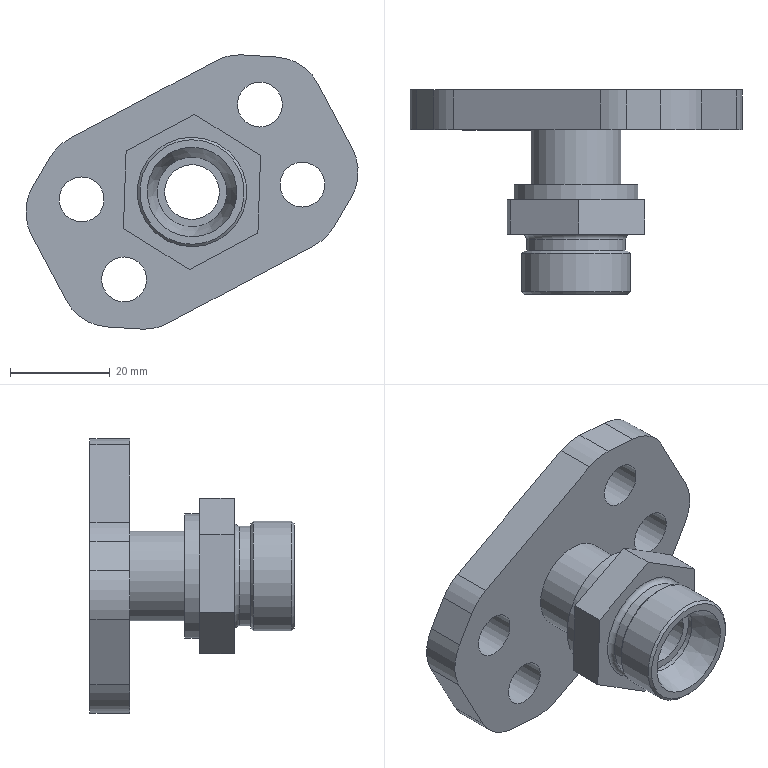Part | STEP file | HL4GZ-1.58.020 (cutter motor inlet/outlet flange) | 2 solids | 54 faces | box 66.692 x 41 x 55.077 mm | volume 25659 mm3 | plane 26 | cylinder 22 | cone 5 | torus 1 | commonest cylinder face diameters 20 x9 9 x4 18 x2 25 x2 11 x1 13 x1